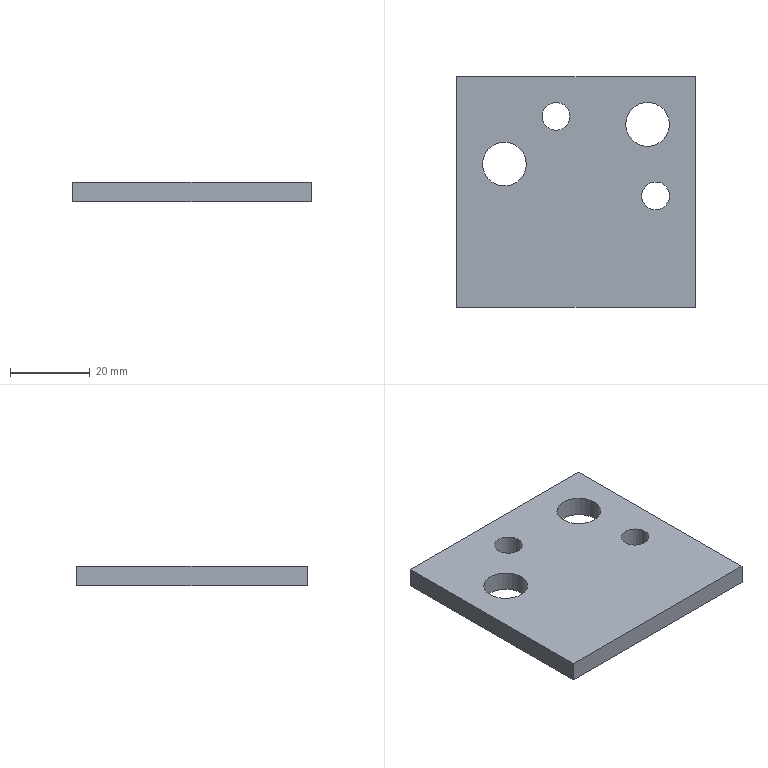Part | NX | features solid 2 | 1 solid | 10 faces | box 60 x 58 x 5 mm | volume 16065 mm3 | plane 6 | cylinder 4 | commonest cylinder face diameters 7 x2 11 x2
STEP:
#1=CARTESIAN_POINT('',(-678.5,-290.,109.));
#2=VERTEX_POINT('',#1);
#3=CARTESIAN_POINT('',(-675.,-290.,109.));
#4=DIRECTION('',(0.,0.,-1.));
#5=DIRECTION('',(-1.,0.,0.));
#6=AXIS2_PLACEMENT_3D('',#3,#4,#5);
#7=CIRCLE('',#6,3.5);
#8=EDGE_CURVE('',#2,#2,#7,.F.);
#9=ORIENTED_EDGE('',*,*,#8,.F.);
#10=EDGE_LOOP('',(#9));
#11=FACE_BOUND('',#10,.T.);
#12=CARTESIAN_POINT('',(-703.5,-270.,109.));
#13=VERTEX_POINT('',#12);
#14=CARTESIAN_POINT('',(-700.,-270.,109.));
#15=DIRECTION('',(0.,0.,-1.));
#16=DIRECTION('',(-1.,0.,0.));
#17=AXIS2_PLACEMENT_3D('',#14,#15,#16);
#18=CIRCLE('',#17,3.5);
#19=EDGE_CURVE('',#13,#13,#18,.F.);
#20=ORIENTED_EDGE('',*,*,#19,.F.);
#21=EDGE_LOOP('',(#20));
#22=FACE_BOUND('',#21,.T.);
#23=CARTESIAN_POINT('',(-682.5,-272.,109.));
#24=VERTEX_POINT('',#23);
#25=CARTESIAN_POINT('',(-677.,-272.,109.));
#26=DIRECTION('',(0.,0.,-1.));
#27=DIRECTION('',(-1.,0.,0.));
#28=AXIS2_PLACEMENT_3D('',#25,#26,#27);
#29=CIRCLE('',#28,5.5);
#30=EDGE_CURVE('',#24,#24,#29,.F.);
#31=ORIENTED_EDGE('',*,*,#30,.F.);
#32=EDGE_LOOP('',(#31));
#33=FACE_BOUND('',#32,.T.);
#34=CARTESIAN_POINT('',(-718.5,-282.,109.));
#35=VERTEX_POINT('',#34);
#36=CARTESIAN_POINT('',(-713.,-282.,109.));
#37=DIRECTION('',(0.,0.,-1.));
#38=DIRECTION('',(-1.,0.,0.));
#39=AXIS2_PLACEMENT_3D('',#36,#37,#38);
#40=CIRCLE('',#39,5.5);
#41=EDGE_CURVE('',#35,#35,#40,.F.);
#42=ORIENTED_EDGE('',*,*,#41,.F.);
#43=EDGE_LOOP('',(#42));
#44=FACE_BOUND('',#43,.T.);
#45=CARTESIAN_POINT('',(-665.,-318.,109.));
#46=VERTEX_POINT('',#45);
#47=CARTESIAN_POINT('',(-665.,-260.,109.));
#48=VERTEX_POINT('',#47);
#49=CARTESIAN_POINT('',(-665.,-260.,109.));
#50=DIRECTION('',(0.,-1.,0.));
#51=VECTOR('',#50,1000.);
#52=LINE('',#49,#51);
#53=EDGE_CURVE('',#46,#48,#52,.F.);
#54=ORIENTED_EDGE('',*,*,#53,.T.);
#55=CARTESIAN_POINT('',(-725.,-260.,109.));
#56=VERTEX_POINT('',#55);
#57=CARTESIAN_POINT('',(-725.,-260.,109.));
#58=DIRECTION('',(1.,0.,0.));
#59=VECTOR('',#58,1000.);
#60=LINE('',#57,#59);
#61=EDGE_CURVE('',#56,#48,#60,.T.);
#62=ORIENTED_EDGE('',*,*,#61,.F.);
#63=CARTESIAN_POINT('',(-725.,-318.,109.));
#64=VERTEX_POINT('',#63);
#65=CARTESIAN_POINT('',(-725.,-260.,109.));
#66=DIRECTION('',(0.,-1.,0.));
#67=VECTOR('',#66,1000.);
#68=LINE('',#65,#67);
#69=EDGE_CURVE('',#64,#56,#68,.F.);
#70=ORIENTED_EDGE('',*,*,#69,.F.);
#71=CARTESIAN_POINT('',(-725.,-318.,109.));
#72=DIRECTION('',(-1.,0.,0.));
#73=VECTOR('',#72,1000.);
#74=LINE('',#71,#73);
#75=EDGE_CURVE('',#64,#46,#74,.F.);
#76=ORIENTED_EDGE('',*,*,#75,.T.);
#77=EDGE_LOOP('',(#54,#62,#70,#76));
#78=FACE_BOUND('',#77,.T.);
#79=CARTESIAN_POINT('',(-725.,-260.,109.));
#80=DIRECTION('',(0.,0.,1.));
#81=DIRECTION('',(1.,0.,0.));
#82=AXIS2_PLACEMENT_3D('',#79,#80,#81);
#83=PLANE('',#82);
#84=ADVANCED_FACE('',(#11,#22,#33,#44,#78),#83,.T.);
#85=ORIENTED_EDGE('',*,*,#69,.T.);
#86=CARTESIAN_POINT('',(-725.,-260.,104.));
#87=VERTEX_POINT('',#86);
#88=CARTESIAN_POINT('',(-725.,-260.,109.));
#89=DIRECTION('',(0.,0.,-1.));
#90=VECTOR('',#89,1000.);
#91=LINE('',#88,#90);
#92=EDGE_CURVE('',#56,#87,#91,.T.);
#93=ORIENTED_EDGE('',*,*,#92,.T.);
#94=CARTESIAN_POINT('',(-725.,-318.,104.));
#95=VERTEX_POINT('',#94);
#96=CARTESIAN_POINT('',(-725.,-260.,104.));
#97=DIRECTION('',(0.,-1.,0.));
#98=VECTOR('',#97,1000.);
#99=LINE('',#96,#98);
#100=EDGE_CURVE('',#95,#87,#99,.F.);
#101=ORIENTED_EDGE('',*,*,#100,.F.);
#102=CARTESIAN_POINT('',(-725.,-318.,0.));
#103=DIRECTION('',(0.,0.,-1.));
#104=VECTOR('',#103,1000.);
#105=LINE('',#102,#104);
#106=EDGE_CURVE('',#64,#95,#105,.T.);
#107=ORIENTED_EDGE('',*,*,#106,.F.);
#108=EDGE_LOOP('',(#85,#93,#101,#107));
#109=FACE_BOUND('',#108,.T.);
#110=CARTESIAN_POINT('',(-725.,-260.,109.));
#111=DIRECTION('',(1.,0.,0.));
#112=DIRECTION('',(0.,0.,-1.));
#113=AXIS2_PLACEMENT_3D('',#110,#111,#112);
#114=PLANE('',#113);
#115=ADVANCED_FACE('',(#109),#114,.F.);
#116=CARTESIAN_POINT('',(-678.5,-290.,104.));
#117=VERTEX_POINT('',#116);
#118=CARTESIAN_POINT('',(-675.,-290.,104.));
#119=DIRECTION('',(0.,0.,-1.));
#120=DIRECTION('',(-1.,0.,0.));
#121=AXIS2_PLACEMENT_3D('',#118,#119,#120);
#122=CIRCLE('',#121,3.5);
#123=EDGE_CURVE('',#117,#117,#122,.T.);
#124=ORIENTED_EDGE('',*,*,#123,.F.);
#125=EDGE_LOOP('',(#124));
#126=FACE_BOUND('',#125,.T.);
#127=CARTESIAN_POINT('',(-703.5,-270.,104.));
#128=VERTEX_POINT('',#127);
#129=CARTESIAN_POINT('',(-700.,-270.,104.));
#130=DIRECTION('',(0.,0.,-1.));
#131=DIRECTION('',(-1.,0.,0.));
#132=AXIS2_PLACEMENT_3D('',#129,#130,#131);
#133=CIRCLE('',#132,3.5);
#134=EDGE_CURVE('',#128,#128,#133,.T.);
#135=ORIENTED_EDGE('',*,*,#134,.F.);
#136=EDGE_LOOP('',(#135));
#137=FACE_BOUND('',#136,.T.);
#138=CARTESIAN_POINT('',(-682.5,-272.,104.));
#139=VERTEX_POINT('',#138);
#140=CARTESIAN_POINT('',(-677.,-272.,104.));
#141=DIRECTION('',(0.,0.,-1.));
#142=DIRECTION('',(-1.,0.,0.));
#143=AXIS2_PLACEMENT_3D('',#140,#141,#142);
#144=CIRCLE('',#143,5.5);
#145=EDGE_CURVE('',#139,#139,#144,.T.);
#146=ORIENTED_EDGE('',*,*,#145,.F.);
#147=EDGE_LOOP('',(#146));
#148=FACE_BOUND('',#147,.T.);
#149=CARTESIAN_POINT('',(-718.5,-282.,104.));
#150=VERTEX_POINT('',#149);
#151=CARTESIAN_POINT('',(-713.,-282.,104.));
#152=DIRECTION('',(0.,0.,-1.));
#153=DIRECTION('',(-1.,0.,0.));
#154=AXIS2_PLACEMENT_3D('',#151,#152,#153);
#155=CIRCLE('',#154,5.5);
#156=EDGE_CURVE('',#150,#150,#155,.T.);
#157=ORIENTED_EDGE('',*,*,#156,.F.);
#158=EDGE_LOOP('',(#157));
#159=FACE_BOUND('',#158,.T.);
#160=ORIENTED_EDGE('',*,*,#100,.T.);
#161=CARTESIAN_POINT('',(-665.,-260.,104.));
#162=VERTEX_POINT('',#161);
#163=CARTESIAN_POINT('',(-725.,-260.,104.));
#164=DIRECTION('',(1.,0.,0.));
#165=VECTOR('',#164,1000.);
#166=LINE('',#163,#165);
#167=EDGE_CURVE('',#87,#162,#166,.T.);
#168=ORIENTED_EDGE('',*,*,#167,.T.);
#169=CARTESIAN_POINT('',(-665.,-318.,104.));
#170=VERTEX_POINT('',#169);
#171=CARTESIAN_POINT('',(-665.,-260.,104.));
#172=DIRECTION('',(0.,-1.,0.));
#173=VECTOR('',#172,1000.);
#174=LINE('',#171,#173);
#175=EDGE_CURVE('',#170,#162,#174,.F.);
#176=ORIENTED_EDGE('',*,*,#175,.F.);
#177=CARTESIAN_POINT('',(0.,-318.,104.));
#178=DIRECTION('',(1.,0.,0.));
#179=VECTOR('',#178,1000.);
#180=LINE('',#177,#179);
#181=EDGE_CURVE('',#95,#170,#180,.T.);
#182=ORIENTED_EDGE('',*,*,#181,.F.);
#183=EDGE_LOOP('',(#160,#168,#176,#182));
#184=FACE_BOUND('',#183,.T.);
#185=CARTESIAN_POINT('',(-725.,-260.,104.));
#186=DIRECTION('',(0.,0.,1.));
#187=DIRECTION('',(1.,0.,0.));
#188=AXIS2_PLACEMENT_3D('',#185,#186,#187);
#189=PLANE('',#188);
#190=ADVANCED_FACE('',(#126,#137,#148,#159,#184),#189,.F.);
#191=CARTESIAN_POINT('',(-665.,-318.,109.));
#192=DIRECTION('',(0.,0.,1.));
#193=VECTOR('',#192,1000.);
#194=LINE('',#191,#193);
#195=EDGE_CURVE('',#46,#170,#194,.F.);
#196=ORIENTED_EDGE('',*,*,#195,.T.);
#197=ORIENTED_EDGE('',*,*,#175,.T.);
#198=CARTESIAN_POINT('',(-665.,-260.,109.));
#199=DIRECTION('',(0.,0.,-1.));
#200=VECTOR('',#199,1000.);
#201=LINE('',#198,#200);
#202=EDGE_CURVE('',#48,#162,#201,.T.);
#203=ORIENTED_EDGE('',*,*,#202,.F.);
#204=ORIENTED_EDGE('',*,*,#53,.F.);
#205=EDGE_LOOP('',(#196,#197,#203,#204));
#206=FACE_BOUND('',#205,.T.);
#207=CARTESIAN_POINT('',(-665.,-260.,109.));
#208=DIRECTION('',(1.,0.,0.));
#209=DIRECTION('',(0.,0.,-1.));
#210=AXIS2_PLACEMENT_3D('',#207,#208,#209);
#211=PLANE('',#210);
#212=ADVANCED_FACE('',(#206),#211,.T.);
#213=ORIENTED_EDGE('',*,*,#167,.F.);
#214=ORIENTED_EDGE('',*,*,#92,.F.);
#215=ORIENTED_EDGE('',*,*,#61,.T.);
#216=ORIENTED_EDGE('',*,*,#202,.T.);
#217=EDGE_LOOP('',(#213,#214,#215,#216));
#218=FACE_BOUND('',#217,.T.);
#219=CARTESIAN_POINT('',(-725.,-260.,109.));
#220=DIRECTION('',(0.,1.,0.));
#221=DIRECTION('',(0.,0.,1.));
#222=AXIS2_PLACEMENT_3D('',#219,#220,#221);
#223=PLANE('',#222);
#224=ADVANCED_FACE('',(#218),#223,.T.);
#225=ORIENTED_EDGE('',*,*,#181,.T.);
#226=ORIENTED_EDGE('',*,*,#195,.F.);
#227=ORIENTED_EDGE('',*,*,#75,.F.);
#228=ORIENTED_EDGE('',*,*,#106,.T.);
#229=EDGE_LOOP('',(#225,#226,#227,#228));
#230=FACE_BOUND('',#229,.T.);
#231=CARTESIAN_POINT('',(0.,-318.,0.));
#232=DIRECTION('',(0.,1.,0.));
#233=DIRECTION('',(0.,0.,1.));
#234=AXIS2_PLACEMENT_3D('',#231,#232,#233);
#235=PLANE('',#234);
#236=ADVANCED_FACE('',(#230),#235,.F.);
#237=ORIENTED_EDGE('',*,*,#156,.T.);
#238=EDGE_LOOP('',(#237));
#239=FACE_BOUND('',#238,.T.);
#240=ORIENTED_EDGE('',*,*,#41,.T.);
#241=EDGE_LOOP('',(#240));
#242=FACE_BOUND('',#241,.T.);
#243=CARTESIAN_POINT('',(-713.,-282.,54.));
#244=DIRECTION('',(0.,0.,1.));
#245=DIRECTION('',(-1.,0.,0.));
#246=AXIS2_PLACEMENT_3D('',#243,#244,#245);
#247=CYLINDRICAL_SURFACE('',#246,5.5);
#248=ADVANCED_FACE('',(#239,#242),#247,.F.);
#249=ORIENTED_EDGE('',*,*,#145,.T.);
#250=EDGE_LOOP('',(#249));
#251=FACE_BOUND('',#250,.T.);
#252=ORIENTED_EDGE('',*,*,#30,.T.);
#253=EDGE_LOOP('',(#252));
#254=FACE_BOUND('',#253,.T.);
#255=CARTESIAN_POINT('',(-677.,-272.,54.));
#256=DIRECTION('',(0.,0.,1.));
#257=DIRECTION('',(-1.,0.,0.));
#258=AXIS2_PLACEMENT_3D('',#255,#256,#257);
#259=CYLINDRICAL_SURFACE('',#258,5.5);
#260=ADVANCED_FACE('',(#251,#254),#259,.F.);
#261=ORIENTED_EDGE('',*,*,#134,.T.);
#262=EDGE_LOOP('',(#261));
#263=FACE_BOUND('',#262,.T.);
#264=ORIENTED_EDGE('',*,*,#19,.T.);
#265=EDGE_LOOP('',(#264));
#266=FACE_BOUND('',#265,.T.);
#267=CARTESIAN_POINT('',(-700.,-270.,54.));
#268=DIRECTION('',(0.,0.,1.));
#269=DIRECTION('',(-1.,0.,0.));
#270=AXIS2_PLACEMENT_3D('',#267,#268,#269);
#271=CYLINDRICAL_SURFACE('',#270,3.5);
#272=ADVANCED_FACE('',(#263,#266),#271,.F.);
#273=ORIENTED_EDGE('',*,*,#123,.T.);
#274=EDGE_LOOP('',(#273));
#275=FACE_BOUND('',#274,.T.);
#276=ORIENTED_EDGE('',*,*,#8,.T.);
#277=EDGE_LOOP('',(#276));
#278=FACE_BOUND('',#277,.T.);
#279=CARTESIAN_POINT('',(-675.,-290.,54.));
#280=DIRECTION('',(0.,0.,1.));
#281=DIRECTION('',(-1.,0.,0.));
#282=AXIS2_PLACEMENT_3D('',#279,#280,#281);
#283=CYLINDRICAL_SURFACE('',#282,3.5);
#284=ADVANCED_FACE('',(#275,#278),#283,.F.);
#285=CLOSED_SHELL('',(#84,#115,#190,#212,#224,#236,#248,#260,#272,#284));
#286=MANIFOLD_SOLID_BREP('',#285);
#287=(LENGTH_UNIT()NAMED_UNIT(*)SI_UNIT(.MILLI.,.METRE.));
#288=UNCERTAINTY_MEASURE_WITH_UNIT(LENGTH_MEASURE(0.00001),#287,'','');
#289=(NAMED_UNIT(*)PLANE_ANGLE_UNIT()SI_UNIT($,.RADIAN.));
#290=(NAMED_UNIT(*)SI_UNIT($,.STERADIAN.)SOLID_ANGLE_UNIT());
#291=(GEOMETRIC_REPRESENTATION_CONTEXT(3)GLOBAL_UNCERTAINTY_ASSIGNED_CONTEXT((#288))GLOBAL_UNIT_ASSIGNED_CONTEXT((#287,#289,#290))REPRESENTATION_CONTEXT('',''));
#292=ADVANCED_BREP_SHAPE_REPRESENTATION('',(#286),#291);